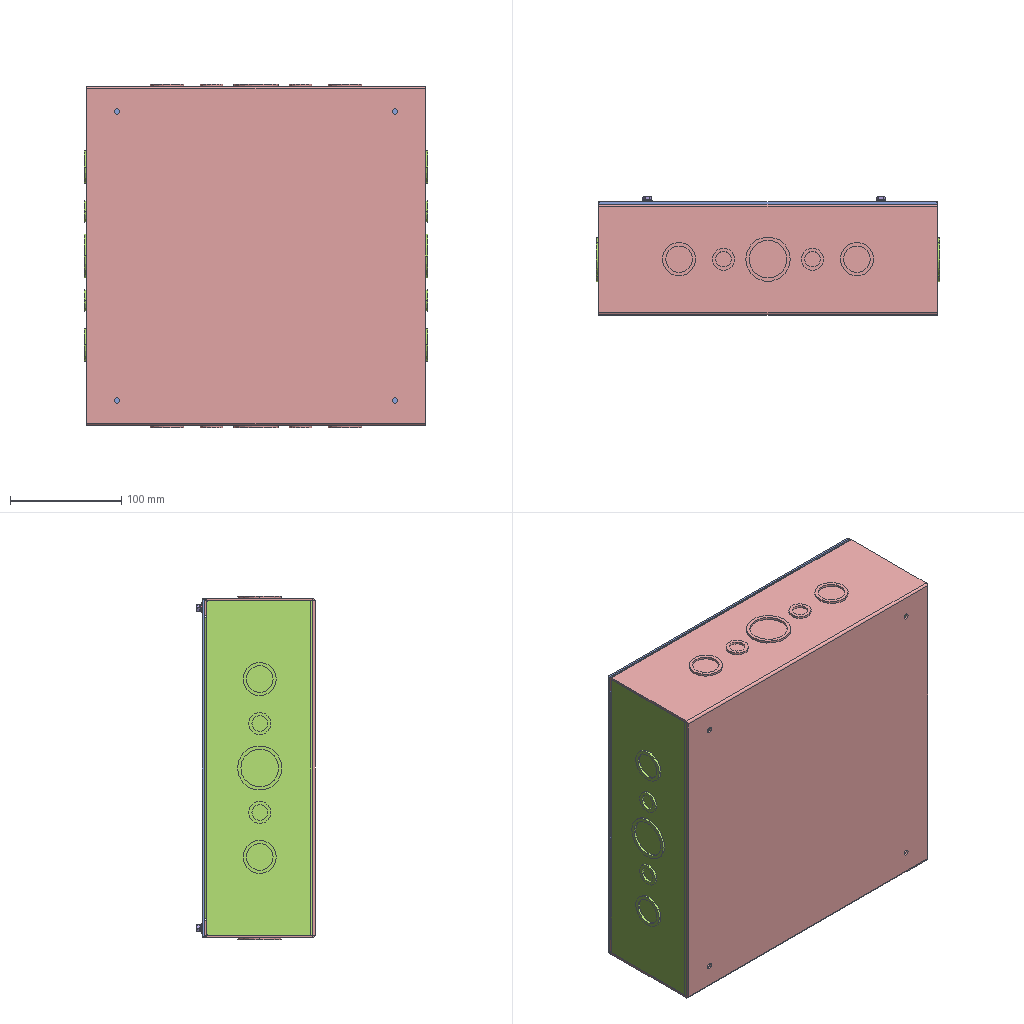Assembly | SolidWorks | 17 different items | 40 placed | box 309 x 106 x 309 mm
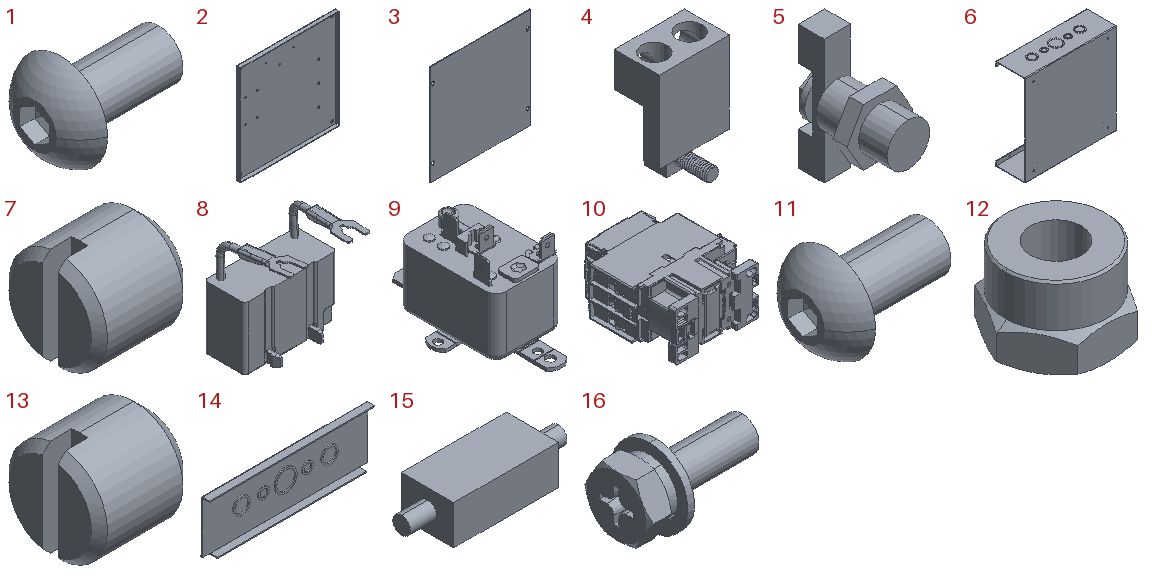Parts list (item | name | quantity | size | volume | features):
1 | - | x1 | 12.75 x 9.5 x 9.5 mm | 311.582 mm3 | features Cut 2, RevCut 2, Boss 1, Extrusion 1, Fillet 1, LPattern 1
2 | - | x1 | 240.001 x 10 x 240.001 mm | 97461 mm3 | features 3DProfileFeature 3, HoleWzd 3, EdgeFlange 1, FlatPattern 1, ICE 1, SMBaseFlange 1, SheetMetal 1
3 | - | x1 | 304.8 x 2 x 304.8 mm | 185210 mm3 | features Fillet 1, FlatPattern 1, ICE 1, LPattern 1, SMBaseFlange 1, SheetMetal 1
4 | - | x3 | 31.72 x 28.25 x 48.96 mm | 13161 mm3 | features ICE 8, Extrusion 1, SweepThread 1
5 | - | x3 | 23.094 x 34.03 x 43.8 mm | 8517 mm3 | features ICE 8, Extrusion 1
6 | - | x1 | 304.8 x 99.6 x 308.8 mm | 331493 mm3 | features ICE 7, EdgeFlange 2, Cut 1, Fillet 1, FlatPattern 1, LPattern 1, SMBaseFlange 1, SheetMetal 1
7 | - | x1 | 10 x 10 x 10 mm | 697.059 mm3 | features Cut 1, LPattern 1, RevCut 1, Revolution 1
8 | - | x1 | 34 x 29.543 x 38.064 mm | 10047 mm3 | features BaseBody 7
9 | - | x1 | 46 x 77 x 40.798 mm | 41564 mm3 | features BaseBody 1
10 | - | x1 | - | - | features BaseBody 56, RefSurface 14, Scale 1
11 | - | x8 | 12.75 x 9.5 x 9.5 mm | 311.582 mm3 | features Cut 2, RevCut 2, Boss 1, Extrusion 1, Fillet 1, LPattern 1
12 | - | x4 | 11.547 x 10 x 8 mm | 473.326 mm3 | features RevCut 3, Boss 1, Chamfer 1, Extrusion 1, LPattern 1
13 | - | x6 | 10 x 10 x 10 mm | 697.059 mm3 | features Cut 1, LPattern 1, RevCut 1, Revolution 1
14 | - | x2 | 300.8 x 17 x 97.6 mm | 77629 mm3 | features EdgeFlange 2, ICE 2, Fillet 1, FlatPattern 1, SMBaseFlange 1, SheetMetal 1
15 | - | x1 | 42 x 14 x 10.5 mm | 3376 mm3 | features ICE 4, Extrusion 1, Scale 1
16 | - | x4 | 14.8 x 9 x 9 mm | 319.757 mm3 | features BaseBody 3
17 | Nut | x1 | - | - | -
Mates (type | each side: item.copy, entity, surface, feature):
Coincident | 6.1 plane | assembly plane | 3 times
Coincident | 6.1 face plane Edge-Flange1 | 3.1 face plane Base-Flange1 | 2 times
Coincident | 6.1 face plane Edge-Flange2 | 3.1 face plane Base-Flange1 | 2 times
Coincident | 6.1 face plane Base-Flange1 | 14.1 face plane Edge-Flange1
Coincident | 6.1 face plane Edge-Flange1 | 14.1 face plane Base-Flange1
Symmetric | 6.1 face plane Edge-Flange1 | 6.1 face plane Edge-Flange1 | 14.1 plane
Coincident | 6.1 face plane Edge-Flange1 | 14.2 face plane Base-Flange1
Coincident | 14.1 face plane Edge-Flange2 | 14.2 face plane Edge-Flange2
Coincident | 14.1 face plane Base-Flange1 | 14.2 face plane Base-Flange1
Symmetric | 6.1 face plane Edge-Flange1 | 6.1 face plane Edge-Flange1 | 2.1 plane
Symmetric | 14.1 face plane Base-Flange1 | 14.2 face plane Base-Flange1 | 2.1 plane
Coincident | 6.1 face plane Base-Flange1 | 2.1 face plane Edge-Flange1
Concentric | 2.1 face cylinder Cut-Extrude1 | 12.1 face cone EndChamfer
Coincident | 2.1 face plane Base-Flange1 | 12.1 face plane BaseNut
Concentric | 2.1 face cylinder Cut-Extrude1 | 12.2 face cone EndChamfer
Coincident | 2.1 face plane Base-Flange1 | 12.2 face plane BaseNut
Concentric | 6.1 face cylinder Boss-Extrude5 | 12.3 face cylinder Extrude1
Concentric | 2.1 face cylinder Cut-Extrude1 | 12.4 face cone EndChamfer
Coincident | 2.1 face plane Base-Flange1 | 12.4 face plane BaseNut
Coincident | 2.1 face plane Base-Flange1 | 12.3 face plane BaseNut
Coincident | 2.1 face plane Base-Flange1 | 15.1 face plane Boss-Extrude1
Concentric | 3.1 face cylinder LPattern1 | 16.1 face cylinder PN_0002 Flat washer grade A ∅4 stainless steel 304 GB.T 97.1-2002-2-solid1
Coincident | 3.1 face plane Base-Flange1 | 16.1 face plane PN_0002 Flat washer grade A ∅4 stainless steel 304 GB.T 97.1-2002-2-solid1
Concentric | 3.1 face cylinder Cut-Extrude1 | 16.2 face cylinder PN_0002 Flat washer grade A ∅4 stainless steel 304 GB.T 97.1-2002-2-solid1
Coincident | 3.1 face plane Base-Flange1 | 16.2 face plane PN_0002 Flat washer grade A ∅4 stainless steel 304 GB.T 97.1-2002-2-solid1
Concentric | 3.1 face cylinder Cut-Extrude1 | 16.3 face cylinder PN_0002 Flat washer grade A ∅4 stainless steel 304 GB.T 97.1-2002-2-solid1
Coincident | 3.1 face plane Base-Flange1 | 16.3 face plane PN_0002 Flat washer grade A ∅4 stainless steel 304 GB.T 97.1-2002-2-solid1
Concentric | 3.1 face cylinder LPattern1 | 16.4 face cylinder PN_0002 Flat washer grade A ∅4 stainless steel 304 GB.T 97.1-2002-2-solid1
Coincident | 3.1 face plane Base-Flange1 | 16.4 face plane PN_0002 Flat washer grade A ∅4 stainless steel 304 GB.T 97.1-2002-2-solid1
Parallel | 14.2 face plane Base-Flange1 | 4.1 face plane Boss-Extrude1
Parallel | 6.1 face plane Edge-Flange1 | 4.1 face plane Boss-Extrude1
Coincident | 2.1 face plane Base-Flange1 | 4.1 face plane Boss-Extrude1
DistanceDim | 4.1 face plane Boss-Extrude1 | 2.1 face plane Edge-Flange1 | 2 times
Concentric | 4.1 face cylinder Cut-Extrude1 | 13.1 face cylinder Base
Concentric | 4.1 face cylinder Cut-Extrude1 | 13.2 face cylinder Base
Coincident | 4.1 face plane Boss-Extrude1 | 13.2 face plane Base
Coincident | 4.1 face plane Boss-Extrude1 | 13.1 face plane Base
Parallel | 2.1 face plane Edge-Flange1 | 10.1 face plane Input 8
Coincident | 2.1 face plane Base-Flange1 | 8.1 face plane Input 2
Parallel | 2.1 face plane Edge-Flange1 | 5.1 face plane Boss-Extrude3
Concentric | 2.1 face cylinder M4 Tapped Hole1 | 11.1 face cylinder BaseBody
Concentric | 2.1 face cylinder M4 Tapped Hole1 | 11.2 face cylinder BaseBody
Concentric | 2.1 face cylinder M4 Tapped Hole1 | 11.3 face cylinder BaseBody
Concentric | 2.1 face cylinder M4 Tapped Hole1 | 11.4 face cylinder BaseBody
Coincident | 11.3 face plane BaseHead | 11.4 face plane BaseHead
Coincident | 11.1 face plane BaseHead | 11.4 face plane BaseHead
Coincident | 11.1 face plane BaseHead | 11.2 face plane BaseHead
Coincident | 10.1 face plane Input 56 | 11.5 face plane BaseHead
Coincident | 11.6 edge | 11.7 face plane BaseHead
Coincident | 11.8 face plane BaseHead | 11.7 face plane BaseHead
Concentric | 10.1 edge | 11.8 face cylinder BaseBody
Coincident | 11.5 edge | 11.8 face plane BaseHead
Concentric | 10.1 face cylinder Input 56 | 11.7 face cylinder BaseBody
Concentric | 10.1 face cylinder Input 56 | 11.6 face cylinder BaseBody
Parallel | 6.1 face plane Edge-Flange1 | 8.1 face plane Input 2
DistanceDim | 5.1 face plane Boss-Extrude4 | 2.1 face plane Base-Flange1